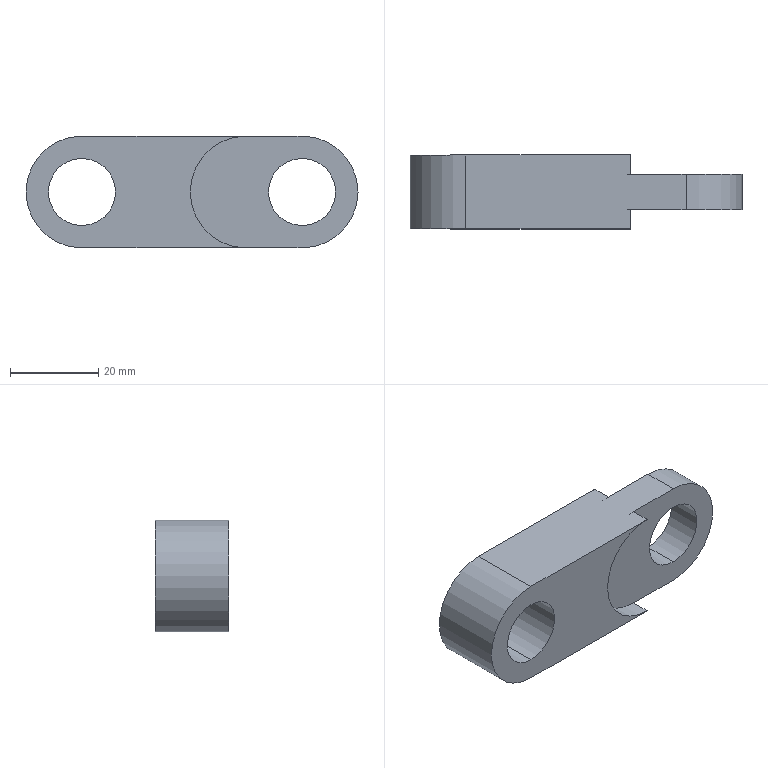Part | SolidWorks | features ICE 3, Extrusion 1, Scale 1 | 1 solid | 14 faces | box 75.4 x 16.764 x 25.4 mm | volume 18082 mm3 | cylinder 8 | plane 6 | commonest cylinder face diameters 15.24 x4 25.4 x4
STEP:
#1=CARTESIAN_POINT('',(0.,16.764,-7.62));
#2=VERTEX_POINT('',#1);
#3=CARTESIAN_POINT('',(0.,16.764,7.62));
#4=VERTEX_POINT('',#3);
#5=CARTESIAN_POINT('',(0.,16.764,0.));
#6=DIRECTION('',(0.,1.,0.));
#7=DIRECTION('',(0.,0.,1.));
#8=AXIS2_PLACEMENT_3D('',#5,#6,#7);
#9=CIRCLE('',#8,7.62);
#10=EDGE_CURVE('',#2,#4,#9,.T.);
#11=ORIENTED_EDGE('',*,*,#10,.T.);
#12=CARTESIAN_POINT('',(0.,0.,7.62));
#13=VERTEX_POINT('',#12);
#14=CARTESIAN_POINT('',(0.,16.764,7.62));
#15=DIRECTION('',(0.,-1.,0.));
#16=VECTOR('',#15,1000.);
#17=LINE('',#14,#16);
#18=EDGE_CURVE('',#4,#13,#17,.T.);
#19=ORIENTED_EDGE('',*,*,#18,.T.);
#20=CARTESIAN_POINT('',(0.,0.,-7.62));
#21=VERTEX_POINT('',#20);
#22=CARTESIAN_POINT('',(0.,0.,0.));
#23=DIRECTION('',(0.,1.,0.));
#24=DIRECTION('',(0.,0.,1.));
#25=AXIS2_PLACEMENT_3D('',#22,#23,#24);
#26=CIRCLE('',#25,7.62);
#27=EDGE_CURVE('',#21,#13,#26,.T.);
#28=ORIENTED_EDGE('',*,*,#27,.F.);
#29=CARTESIAN_POINT('',(0.,16.764,-7.62));
#30=DIRECTION('',(0.,-1.,0.));
#31=VECTOR('',#30,1000.);
#32=LINE('',#29,#31);
#33=EDGE_CURVE('',#2,#21,#32,.T.);
#34=ORIENTED_EDGE('',*,*,#33,.F.);
#35=EDGE_LOOP('',(#11,#19,#28,#34));
#36=FACE_OUTER_BOUND('',#35,.T.);
#37=CARTESIAN_POINT('',(0.,16.764,0.));
#38=DIRECTION('',(0.,-1.,0.));
#39=DIRECTION('',(0.,0.,-1.));
#40=AXIS2_PLACEMENT_3D('',#37,#38,#39);
#41=CYLINDRICAL_SURFACE('',#40,7.62);
#42=ADVANCED_FACE('',(#36),#41,.F.);
#43=CARTESIAN_POINT('',(50.,12.446,7.62));
#44=VERTEX_POINT('',#43);
#45=CARTESIAN_POINT('',(50.,12.446,-7.62));
#46=VERTEX_POINT('',#45);
#47=CARTESIAN_POINT('',(50.,12.446,0.));
#48=DIRECTION('',(0.,-1.,0.));
#49=DIRECTION('',(0.,0.,-1.));
#50=AXIS2_PLACEMENT_3D('',#47,#48,#49);
#51=CIRCLE('',#50,7.62);
#52=EDGE_CURVE('',#44,#46,#51,.T.);
#53=ORIENTED_EDGE('',*,*,#52,.F.);
#54=CARTESIAN_POINT('',(50.,4.318,7.62));
#55=VERTEX_POINT('',#54);
#56=CARTESIAN_POINT('',(50.,16.764,7.62));
#57=DIRECTION('',(0.,-1.,0.));
#58=VECTOR('',#57,1000.);
#59=LINE('',#56,#58);
#60=EDGE_CURVE('',#44,#55,#59,.T.);
#61=ORIENTED_EDGE('',*,*,#60,.T.);
#62=CARTESIAN_POINT('',(50.,4.318,-7.62));
#63=VERTEX_POINT('',#62);
#64=CARTESIAN_POINT('',(50.,4.318,0.));
#65=DIRECTION('',(0.,-1.,0.));
#66=DIRECTION('',(0.,0.,-1.));
#67=AXIS2_PLACEMENT_3D('',#64,#65,#66);
#68=CIRCLE('',#67,7.62);
#69=EDGE_CURVE('',#55,#63,#68,.T.);
#70=ORIENTED_EDGE('',*,*,#69,.T.);
#71=CARTESIAN_POINT('',(50.,16.764,-7.62));
#72=DIRECTION('',(0.,-1.,0.));
#73=VECTOR('',#72,1000.);
#74=LINE('',#71,#73);
#75=EDGE_CURVE('',#46,#63,#74,.T.);
#76=ORIENTED_EDGE('',*,*,#75,.F.);
#77=EDGE_LOOP('',(#53,#61,#70,#76));
#78=FACE_OUTER_BOUND('',#77,.T.);
#79=CARTESIAN_POINT('',(50.,16.764,0.));
#80=DIRECTION('',(0.,-1.,0.));
#81=DIRECTION('',(0.,0.,-1.));
#82=AXIS2_PLACEMENT_3D('',#79,#80,#81);
#83=CYLINDRICAL_SURFACE('',#82,7.62);
#84=ADVANCED_FACE('',(#78),#83,.F.);
#85=CARTESIAN_POINT('',(50.,12.446,-12.7));
#86=VERTEX_POINT('',#85);
#87=CARTESIAN_POINT('',(50.,4.318,-12.7));
#88=VERTEX_POINT('',#87);
#89=CARTESIAN_POINT('',(50.,16.764,-12.7));
#90=DIRECTION('',(0.,-1.,0.));
#91=VECTOR('',#90,1000.);
#92=LINE('',#89,#91);
#93=EDGE_CURVE('',#86,#88,#92,.T.);
#94=ORIENTED_EDGE('',*,*,#93,.F.);
#95=CARTESIAN_POINT('',(50.,12.446,12.7));
#96=VERTEX_POINT('',#95);
#97=CARTESIAN_POINT('',(50.,12.446,0.));
#98=DIRECTION('',(0.,-1.,0.));
#99=DIRECTION('',(0.,0.,-1.));
#100=AXIS2_PLACEMENT_3D('',#97,#98,#99);
#101=CIRCLE('',#100,12.7);
#102=EDGE_CURVE('',#86,#96,#101,.T.);
#103=ORIENTED_EDGE('',*,*,#102,.T.);
#104=CARTESIAN_POINT('',(50.,4.318,12.7));
#105=VERTEX_POINT('',#104);
#106=CARTESIAN_POINT('',(50.,16.764,12.7));
#107=DIRECTION('',(0.,-1.,0.));
#108=VECTOR('',#107,1000.);
#109=LINE('',#106,#108);
#110=EDGE_CURVE('',#96,#105,#109,.T.);
#111=ORIENTED_EDGE('',*,*,#110,.T.);
#112=CARTESIAN_POINT('',(50.,4.318,0.));
#113=DIRECTION('',(0.,-1.,0.));
#114=DIRECTION('',(0.,0.,-1.));
#115=AXIS2_PLACEMENT_3D('',#112,#113,#114);
#116=CIRCLE('',#115,12.7);
#117=EDGE_CURVE('',#88,#105,#116,.T.);
#118=ORIENTED_EDGE('',*,*,#117,.F.);
#119=EDGE_LOOP('',(#94,#103,#111,#118));
#120=FACE_OUTER_BOUND('',#119,.T.);
#121=CARTESIAN_POINT('',(50.,16.764,0.));
#122=DIRECTION('',(0.,-1.,0.));
#123=DIRECTION('',(0.,0.,-1.));
#124=AXIS2_PLACEMENT_3D('',#121,#122,#123);
#125=CYLINDRICAL_SURFACE('',#124,12.7);
#126=ADVANCED_FACE('',(#120),#125,.T.);
#127=ORIENTED_EDGE('',*,*,#60,.F.);
#128=CARTESIAN_POINT('',(50.,12.446,0.));
#129=DIRECTION('',(0.,-1.,0.));
#130=DIRECTION('',(0.,0.,-1.));
#131=AXIS2_PLACEMENT_3D('',#128,#129,#130);
#132=CIRCLE('',#131,7.62);
#133=EDGE_CURVE('',#46,#44,#132,.T.);
#134=ORIENTED_EDGE('',*,*,#133,.F.);
#135=ORIENTED_EDGE('',*,*,#75,.T.);
#136=CARTESIAN_POINT('',(50.,4.318,0.));
#137=DIRECTION('',(0.,-1.,0.));
#138=DIRECTION('',(0.,0.,-1.));
#139=AXIS2_PLACEMENT_3D('',#136,#137,#138);
#140=CIRCLE('',#139,7.62);
#141=EDGE_CURVE('',#63,#55,#140,.T.);
#142=ORIENTED_EDGE('',*,*,#141,.T.);
#143=EDGE_LOOP('',(#127,#134,#135,#142));
#144=FACE_OUTER_BOUND('',#143,.T.);
#145=CARTESIAN_POINT('',(50.,16.764,0.));
#146=DIRECTION('',(0.,-1.,0.));
#147=DIRECTION('',(0.,0.,-1.));
#148=AXIS2_PLACEMENT_3D('',#145,#146,#147);
#149=CYLINDRICAL_SURFACE('',#148,7.62);
#150=ADVANCED_FACE('',(#144),#149,.F.);
#151=CARTESIAN_POINT('',(37.3,16.764,-12.7));
#152=VERTEX_POINT('',#151);
#153=CARTESIAN_POINT('',(37.3,16.764,12.7));
#154=VERTEX_POINT('',#153);
#155=CARTESIAN_POINT('',(37.3,16.764,0.));
#156=DIRECTION('',(0.,1.,0.));
#157=DIRECTION('',(0.,0.,1.));
#158=AXIS2_PLACEMENT_3D('',#155,#156,#157);
#159=CIRCLE('',#158,12.7);
#160=EDGE_CURVE('',#152,#154,#159,.T.);
#161=ORIENTED_EDGE('',*,*,#160,.F.);
#162=CARTESIAN_POINT('',(0.,16.764,-12.7));
#163=VERTEX_POINT('',#162);
#164=CARTESIAN_POINT('',(0.,16.764,-12.7));
#165=DIRECTION('',(-1.,0.,0.));
#166=VECTOR('',#165,1000.);
#167=LINE('',#164,#166);
#168=EDGE_CURVE('',#152,#163,#167,.T.);
#169=ORIENTED_EDGE('',*,*,#168,.T.);
#170=CARTESIAN_POINT('',(0.,16.764,12.7));
#171=VERTEX_POINT('',#170);
#172=CARTESIAN_POINT('',(0.,16.764,0.));
#173=DIRECTION('',(0.,1.,0.));
#174=DIRECTION('',(0.,0.,1.));
#175=AXIS2_PLACEMENT_3D('',#172,#173,#174);
#176=CIRCLE('',#175,12.7);
#177=EDGE_CURVE('',#163,#171,#176,.T.);
#178=ORIENTED_EDGE('',*,*,#177,.T.);
#179=CARTESIAN_POINT('',(0.,16.764,12.7));
#180=DIRECTION('',(1.,0.,0.));
#181=VECTOR('',#180,1000.);
#182=LINE('',#179,#181);
#183=EDGE_CURVE('',#171,#154,#182,.T.);
#184=ORIENTED_EDGE('',*,*,#183,.T.);
#185=EDGE_LOOP('',(#161,#169,#178,#184));
#186=FACE_OUTER_BOUND('',#185,.T.);
#187=ORIENTED_EDGE('',*,*,#10,.F.);
#188=CARTESIAN_POINT('',(0.,16.764,0.));
#189=DIRECTION('',(0.,1.,0.));
#190=DIRECTION('',(0.,0.,1.));
#191=AXIS2_PLACEMENT_3D('',#188,#189,#190);
#192=CIRCLE('',#191,7.62);
#193=EDGE_CURVE('',#4,#2,#192,.T.);
#194=ORIENTED_EDGE('',*,*,#193,.F.);
#195=EDGE_LOOP('',(#187,#194));
#196=FACE_BOUND('',#195,.T.);
#197=CARTESIAN_POINT('',(0.,16.764,0.));
#198=DIRECTION('',(0.,1.,0.));
#199=DIRECTION('',(0.,0.,1.));
#200=AXIS2_PLACEMENT_3D('',#197,#198,#199);
#201=PLANE('',#200);
#202=ADVANCED_FACE('',(#186,#196),#201,.T.);
#203=CARTESIAN_POINT('',(37.3,0.,-12.7));
#204=VERTEX_POINT('',#203);
#205=CARTESIAN_POINT('',(0.,0.,-12.7));
#206=VERTEX_POINT('',#205);
#207=CARTESIAN_POINT('',(0.,0.,-12.7));
#208=DIRECTION('',(-1.,0.,0.));
#209=VECTOR('',#208,1000.);
#210=LINE('',#207,#209);
#211=EDGE_CURVE('',#204,#206,#210,.T.);
#212=ORIENTED_EDGE('',*,*,#211,.F.);
#213=CARTESIAN_POINT('',(37.3,0.,12.7));
#214=VERTEX_POINT('',#213);
#215=CARTESIAN_POINT('',(37.3,0.,0.));
#216=DIRECTION('',(0.,-1.,0.));
#217=DIRECTION('',(0.,0.,-1.));
#218=AXIS2_PLACEMENT_3D('',#215,#216,#217);
#219=CIRCLE('',#218,12.7);
#220=EDGE_CURVE('',#214,#204,#219,.T.);
#221=ORIENTED_EDGE('',*,*,#220,.F.);
#222=CARTESIAN_POINT('',(0.,0.,12.7));
#223=VERTEX_POINT('',#222);
#224=CARTESIAN_POINT('',(0.,0.,12.7));
#225=DIRECTION('',(1.,0.,0.));
#226=VECTOR('',#225,1000.);
#227=LINE('',#224,#226);
#228=EDGE_CURVE('',#223,#214,#227,.T.);
#229=ORIENTED_EDGE('',*,*,#228,.F.);
#230=CARTESIAN_POINT('',(0.,0.,0.));
#231=DIRECTION('',(0.,1.,0.));
#232=DIRECTION('',(0.,0.,1.));
#233=AXIS2_PLACEMENT_3D('',#230,#231,#232);
#234=CIRCLE('',#233,12.7);
#235=EDGE_CURVE('',#206,#223,#234,.T.);
#236=ORIENTED_EDGE('',*,*,#235,.F.);
#237=EDGE_LOOP('',(#212,#221,#229,#236));
#238=FACE_OUTER_BOUND('',#237,.T.);
#239=ORIENTED_EDGE('',*,*,#27,.T.);
#240=CARTESIAN_POINT('',(0.,0.,0.));
#241=DIRECTION('',(0.,1.,0.));
#242=DIRECTION('',(0.,0.,1.));
#243=AXIS2_PLACEMENT_3D('',#240,#241,#242);
#244=CIRCLE('',#243,7.62);
#245=EDGE_CURVE('',#13,#21,#244,.T.);
#246=ORIENTED_EDGE('',*,*,#245,.T.);
#247=EDGE_LOOP('',(#239,#246));
#248=FACE_BOUND('',#247,.T.);
#249=CARTESIAN_POINT('',(0.,0.,0.));
#250=DIRECTION('',(0.,1.,0.));
#251=DIRECTION('',(0.,0.,1.));
#252=AXIS2_PLACEMENT_3D('',#249,#250,#251);
#253=PLANE('',#252);
#254=ADVANCED_FACE('',(#238,#248),#253,.F.);
#255=ORIENTED_EDGE('',*,*,#235,.T.);
#256=CARTESIAN_POINT('',(0.,16.764,12.7));
#257=DIRECTION('',(0.,-1.,0.));
#258=VECTOR('',#257,1000.);
#259=LINE('',#256,#258);
#260=EDGE_CURVE('',#171,#223,#259,.T.);
#261=ORIENTED_EDGE('',*,*,#260,.F.);
#262=ORIENTED_EDGE('',*,*,#177,.F.);
#263=CARTESIAN_POINT('',(0.,16.764,-12.7));
#264=DIRECTION('',(0.,-1.,0.));
#265=VECTOR('',#264,1000.);
#266=LINE('',#263,#265);
#267=EDGE_CURVE('',#163,#206,#266,.T.);
#268=ORIENTED_EDGE('',*,*,#267,.T.);
#269=EDGE_LOOP('',(#255,#261,#262,#268));
#270=FACE_OUTER_BOUND('',#269,.T.);
#271=CARTESIAN_POINT('',(0.,16.764,0.));
#272=DIRECTION('',(0.,-1.,0.));
#273=DIRECTION('',(0.,0.,-1.));
#274=AXIS2_PLACEMENT_3D('',#271,#272,#273);
#275=CYLINDRICAL_SURFACE('',#274,12.7);
#276=ADVANCED_FACE('',(#270),#275,.T.);
#277=ORIENTED_EDGE('',*,*,#110,.F.);
#278=CARTESIAN_POINT('',(37.3,12.446,12.7));
#279=VERTEX_POINT('',#278);
#280=CARTESIAN_POINT('',(0.,12.446,12.7));
#281=DIRECTION('',(1.,0.,0.));
#282=VECTOR('',#281,1000.);
#283=LINE('',#280,#282);
#284=EDGE_CURVE('',#279,#96,#283,.T.);
#285=ORIENTED_EDGE('',*,*,#284,.F.);
#286=CARTESIAN_POINT('',(37.3,0.,12.7));
#287=DIRECTION('',(0.,-1.,0.));
#288=VECTOR('',#287,1000.);
#289=LINE('',#286,#288);
#290=EDGE_CURVE('',#154,#279,#289,.T.);
#291=ORIENTED_EDGE('',*,*,#290,.F.);
#292=ORIENTED_EDGE('',*,*,#183,.F.);
#293=ORIENTED_EDGE('',*,*,#260,.T.);
#294=ORIENTED_EDGE('',*,*,#228,.T.);
#295=CARTESIAN_POINT('',(37.3,4.318,12.7));
#296=VERTEX_POINT('',#295);
#297=CARTESIAN_POINT('',(37.3,0.,12.7));
#298=DIRECTION('',(0.,-1.,0.));
#299=VECTOR('',#298,1000.);
#300=LINE('',#297,#299);
#301=EDGE_CURVE('',#296,#214,#300,.T.);
#302=ORIENTED_EDGE('',*,*,#301,.F.);
#303=CARTESIAN_POINT('',(0.,4.318,12.7));
#304=DIRECTION('',(1.,0.,0.));
#305=VECTOR('',#304,1000.);
#306=LINE('',#303,#305);
#307=EDGE_CURVE('',#296,#105,#306,.T.);
#308=ORIENTED_EDGE('',*,*,#307,.T.);
#309=EDGE_LOOP('',(#277,#285,#291,#292,#293,#294,#302,#308));
#310=FACE_OUTER_BOUND('',#309,.T.);
#311=CARTESIAN_POINT('',(0.,16.764,12.7));
#312=DIRECTION('',(0.,0.,-1.));
#313=DIRECTION('',(-1.,0.,0.));
#314=AXIS2_PLACEMENT_3D('',#311,#312,#313);
#315=PLANE('',#314);
#316=ADVANCED_FACE('',(#310),#315,.F.);
#317=CARTESIAN_POINT('',(37.3,12.446,-12.7));
#318=VERTEX_POINT('',#317);
#319=CARTESIAN_POINT('',(37.3,0.,-12.7));
#320=DIRECTION('',(0.,-1.,0.));
#321=VECTOR('',#320,1000.);
#322=LINE('',#319,#321);
#323=EDGE_CURVE('',#152,#318,#322,.T.);
#324=ORIENTED_EDGE('',*,*,#323,.T.);
#325=CARTESIAN_POINT('',(0.,12.446,-12.7));
#326=DIRECTION('',(1.,0.,0.));
#327=VECTOR('',#326,1000.);
#328=LINE('',#325,#327);
#329=EDGE_CURVE('',#318,#86,#328,.T.);
#330=ORIENTED_EDGE('',*,*,#329,.T.);
#331=ORIENTED_EDGE('',*,*,#93,.T.);
#332=CARTESIAN_POINT('',(37.3,4.318,-12.7));
#333=VERTEX_POINT('',#332);
#334=CARTESIAN_POINT('',(0.,4.318,-12.7));
#335=DIRECTION('',(1.,0.,0.));
#336=VECTOR('',#335,1000.);
#337=LINE('',#334,#336);
#338=EDGE_CURVE('',#333,#88,#337,.T.);
#339=ORIENTED_EDGE('',*,*,#338,.F.);
#340=CARTESIAN_POINT('',(37.3,0.,-12.7));
#341=DIRECTION('',(0.,-1.,0.));
#342=VECTOR('',#341,1000.);
#343=LINE('',#340,#342);
#344=EDGE_CURVE('',#333,#204,#343,.T.);
#345=ORIENTED_EDGE('',*,*,#344,.T.);
#346=ORIENTED_EDGE('',*,*,#211,.T.);
#347=ORIENTED_EDGE('',*,*,#267,.F.);
#348=ORIENTED_EDGE('',*,*,#168,.F.);
#349=EDGE_LOOP('',(#324,#330,#331,#339,#345,#346,#347,#348));
#350=FACE_OUTER_BOUND('',#349,.T.);
#351=CARTESIAN_POINT('',(0.,16.764,-12.7));
#352=DIRECTION('',(0.,0.,1.));
#353=DIRECTION('',(1.,0.,0.));
#354=AXIS2_PLACEMENT_3D('',#351,#352,#353);
#355=PLANE('',#354);
#356=ADVANCED_FACE('',(#350),#355,.F.);
#357=ORIENTED_EDGE('',*,*,#18,.F.);
#358=ORIENTED_EDGE('',*,*,#193,.T.);
#359=ORIENTED_EDGE('',*,*,#33,.T.);
#360=ORIENTED_EDGE('',*,*,#245,.F.);
#361=EDGE_LOOP('',(#357,#358,#359,#360));
#362=FACE_OUTER_BOUND('',#361,.T.);
#363=CARTESIAN_POINT('',(0.,16.764,0.));
#364=DIRECTION('',(0.,-1.,0.));
#365=DIRECTION('',(0.,0.,-1.));
#366=AXIS2_PLACEMENT_3D('',#363,#364,#365);
#367=CYLINDRICAL_SURFACE('',#366,7.62);
#368=ADVANCED_FACE('',(#362),#367,.F.);
#369=ORIENTED_EDGE('',*,*,#141,.F.);
#370=ORIENTED_EDGE('',*,*,#69,.F.);
#371=EDGE_LOOP('',(#369,#370));
#372=FACE_BOUND('',#371,.T.);
#373=CARTESIAN_POINT('',(37.3,4.318,0.));
#374=DIRECTION('',(0.,1.,0.));
#375=DIRECTION('',(0.,0.,-1.));
#376=AXIS2_PLACEMENT_3D('',#373,#374,#375);
#377=CIRCLE('',#376,12.7);
#378=EDGE_CURVE('',#333,#296,#377,.T.);
#379=ORIENTED_EDGE('',*,*,#378,.F.);
#380=ORIENTED_EDGE('',*,*,#338,.T.);
#381=ORIENTED_EDGE('',*,*,#117,.T.);
#382=ORIENTED_EDGE('',*,*,#307,.F.);
#383=EDGE_LOOP('',(#379,#380,#381,#382));
#384=FACE_OUTER_BOUND('',#383,.T.);
#385=CARTESIAN_POINT('',(0.,4.318,-12.7));
#386=DIRECTION('',(0.,-1.,0.));
#387=DIRECTION('',(0.,0.,-1.));
#388=AXIS2_PLACEMENT_3D('',#385,#386,#387);
#389=PLANE('',#388);
#390=ADVANCED_FACE('',(#372,#384),#389,.T.);
#391=ORIENTED_EDGE('',*,*,#133,.T.);
#392=ORIENTED_EDGE('',*,*,#52,.T.);
#393=EDGE_LOOP('',(#391,#392));
#394=FACE_BOUND('',#393,.T.);
#395=ORIENTED_EDGE('',*,*,#329,.F.);
#396=CARTESIAN_POINT('',(37.3,12.446,0.));
#397=DIRECTION('',(0.,1.,0.));
#398=DIRECTION('',(0.,0.,-1.));
#399=AXIS2_PLACEMENT_3D('',#396,#397,#398);
#400=CIRCLE('',#399,12.7);
#401=EDGE_CURVE('',#318,#279,#400,.T.);
#402=ORIENTED_EDGE('',*,*,#401,.T.);
#403=ORIENTED_EDGE('',*,*,#284,.T.);
#404=ORIENTED_EDGE('',*,*,#102,.F.);
#405=EDGE_LOOP('',(#395,#402,#403,#404));
#406=FACE_OUTER_BOUND('',#405,.T.);
#407=CARTESIAN_POINT('',(0.,12.446,-12.7));
#408=DIRECTION('',(0.,-1.,0.));
#409=DIRECTION('',(0.,0.,-1.));
#410=AXIS2_PLACEMENT_3D('',#407,#408,#409);
#411=PLANE('',#410);
#412=ADVANCED_FACE('',(#394,#406),#411,.F.);
#413=ORIENTED_EDGE('',*,*,#378,.T.);
#414=ORIENTED_EDGE('',*,*,#301,.T.);
#415=ORIENTED_EDGE('',*,*,#220,.T.);
#416=ORIENTED_EDGE('',*,*,#344,.F.);
#417=EDGE_LOOP('',(#413,#414,#415,#416));
#418=FACE_OUTER_BOUND('',#417,.T.);
#419=CARTESIAN_POINT('',(37.3,40.239,0.));
#420=DIRECTION('',(0.,-1.,0.));
#421=DIRECTION('',(0.,0.,-1.));
#422=AXIS2_PLACEMENT_3D('',#419,#420,#421);
#423=CYLINDRICAL_SURFACE('',#422,12.7);
#424=ADVANCED_FACE('',(#418),#423,.F.);
#425=ORIENTED_EDGE('',*,*,#401,.F.);
#426=ORIENTED_EDGE('',*,*,#323,.F.);
#427=ORIENTED_EDGE('',*,*,#160,.T.);
#428=ORIENTED_EDGE('',*,*,#290,.T.);
#429=EDGE_LOOP('',(#425,#426,#427,#428));
#430=FACE_OUTER_BOUND('',#429,.T.);
#431=CARTESIAN_POINT('',(37.3,-23.475,0.));
#432=DIRECTION('',(0.,1.,0.));
#433=DIRECTION('',(0.,0.,1.));
#434=AXIS2_PLACEMENT_3D('',#431,#432,#433);
#435=CYLINDRICAL_SURFACE('',#434,12.7);
#436=ADVANCED_FACE('',(#430),#435,.F.);
#437=CLOSED_SHELL('',(#42,#84,#126,#150,#202,#254,#276,#316,#356,#368,#390,#412,#424,#436));
#438=MANIFOLD_SOLID_BREP('',#437);
#439=CARTESIAN_POINT('',(0.,0.,0.));
#440=DIRECTION('',(0.,0.,1.));
#441=DIRECTION('',(1.,0.,0.));
#442=AXIS2_PLACEMENT_3D('',#439,#440,#441);
#443=(LENGTH_UNIT()NAMED_UNIT(*)SI_UNIT(.MILLI.,.METRE.));
#444=UNCERTAINTY_MEASURE_WITH_UNIT(LENGTH_MEASURE(0.00001),#443,'','');
#445=(NAMED_UNIT(*)PLANE_ANGLE_UNIT()SI_UNIT($,.RADIAN.));
#446=(NAMED_UNIT(*)SI_UNIT($,.STERADIAN.)SOLID_ANGLE_UNIT());
#447=(GEOMETRIC_REPRESENTATION_CONTEXT(3)GLOBAL_UNCERTAINTY_ASSIGNED_CONTEXT((#444))GLOBAL_UNIT_ASSIGNED_CONTEXT((#443,#445,#446))REPRESENTATION_CONTEXT('',''));
#448=ADVANCED_BREP_SHAPE_REPRESENTATION('',(#438,#442),#447);